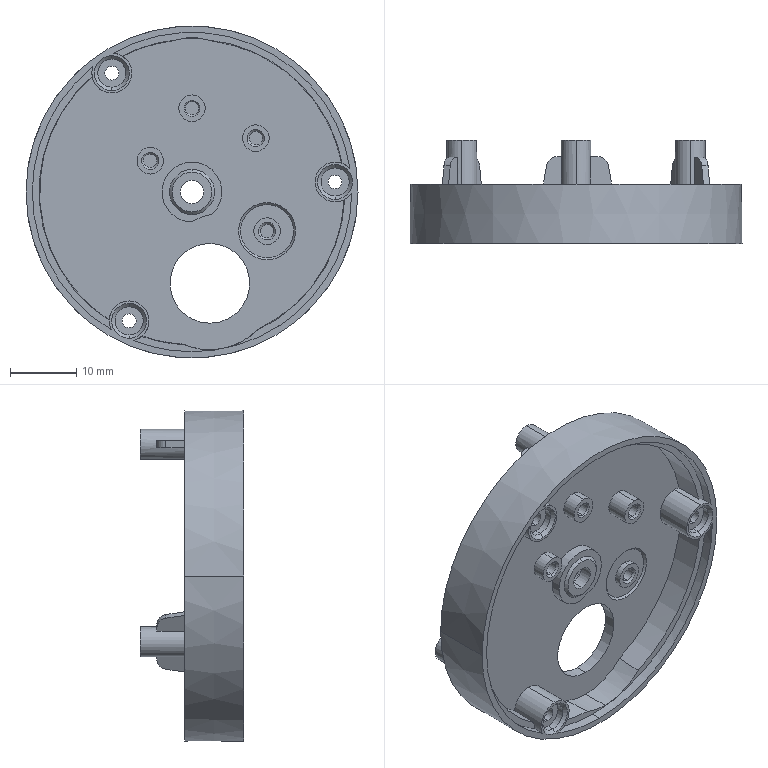Part | SolidWorks | features BaseBody 1 | 1 solid | 224 faces | box 49.947 x 15.55 x 49.947 mm | volume 5586 mm3 | cylinder 88 | plane 87 | cone 44 | spline 5 | commonest cylinder face diameters 4 x11 5.95 x11 2.02 x8 2 x6 2.1 x6 3.26 x6